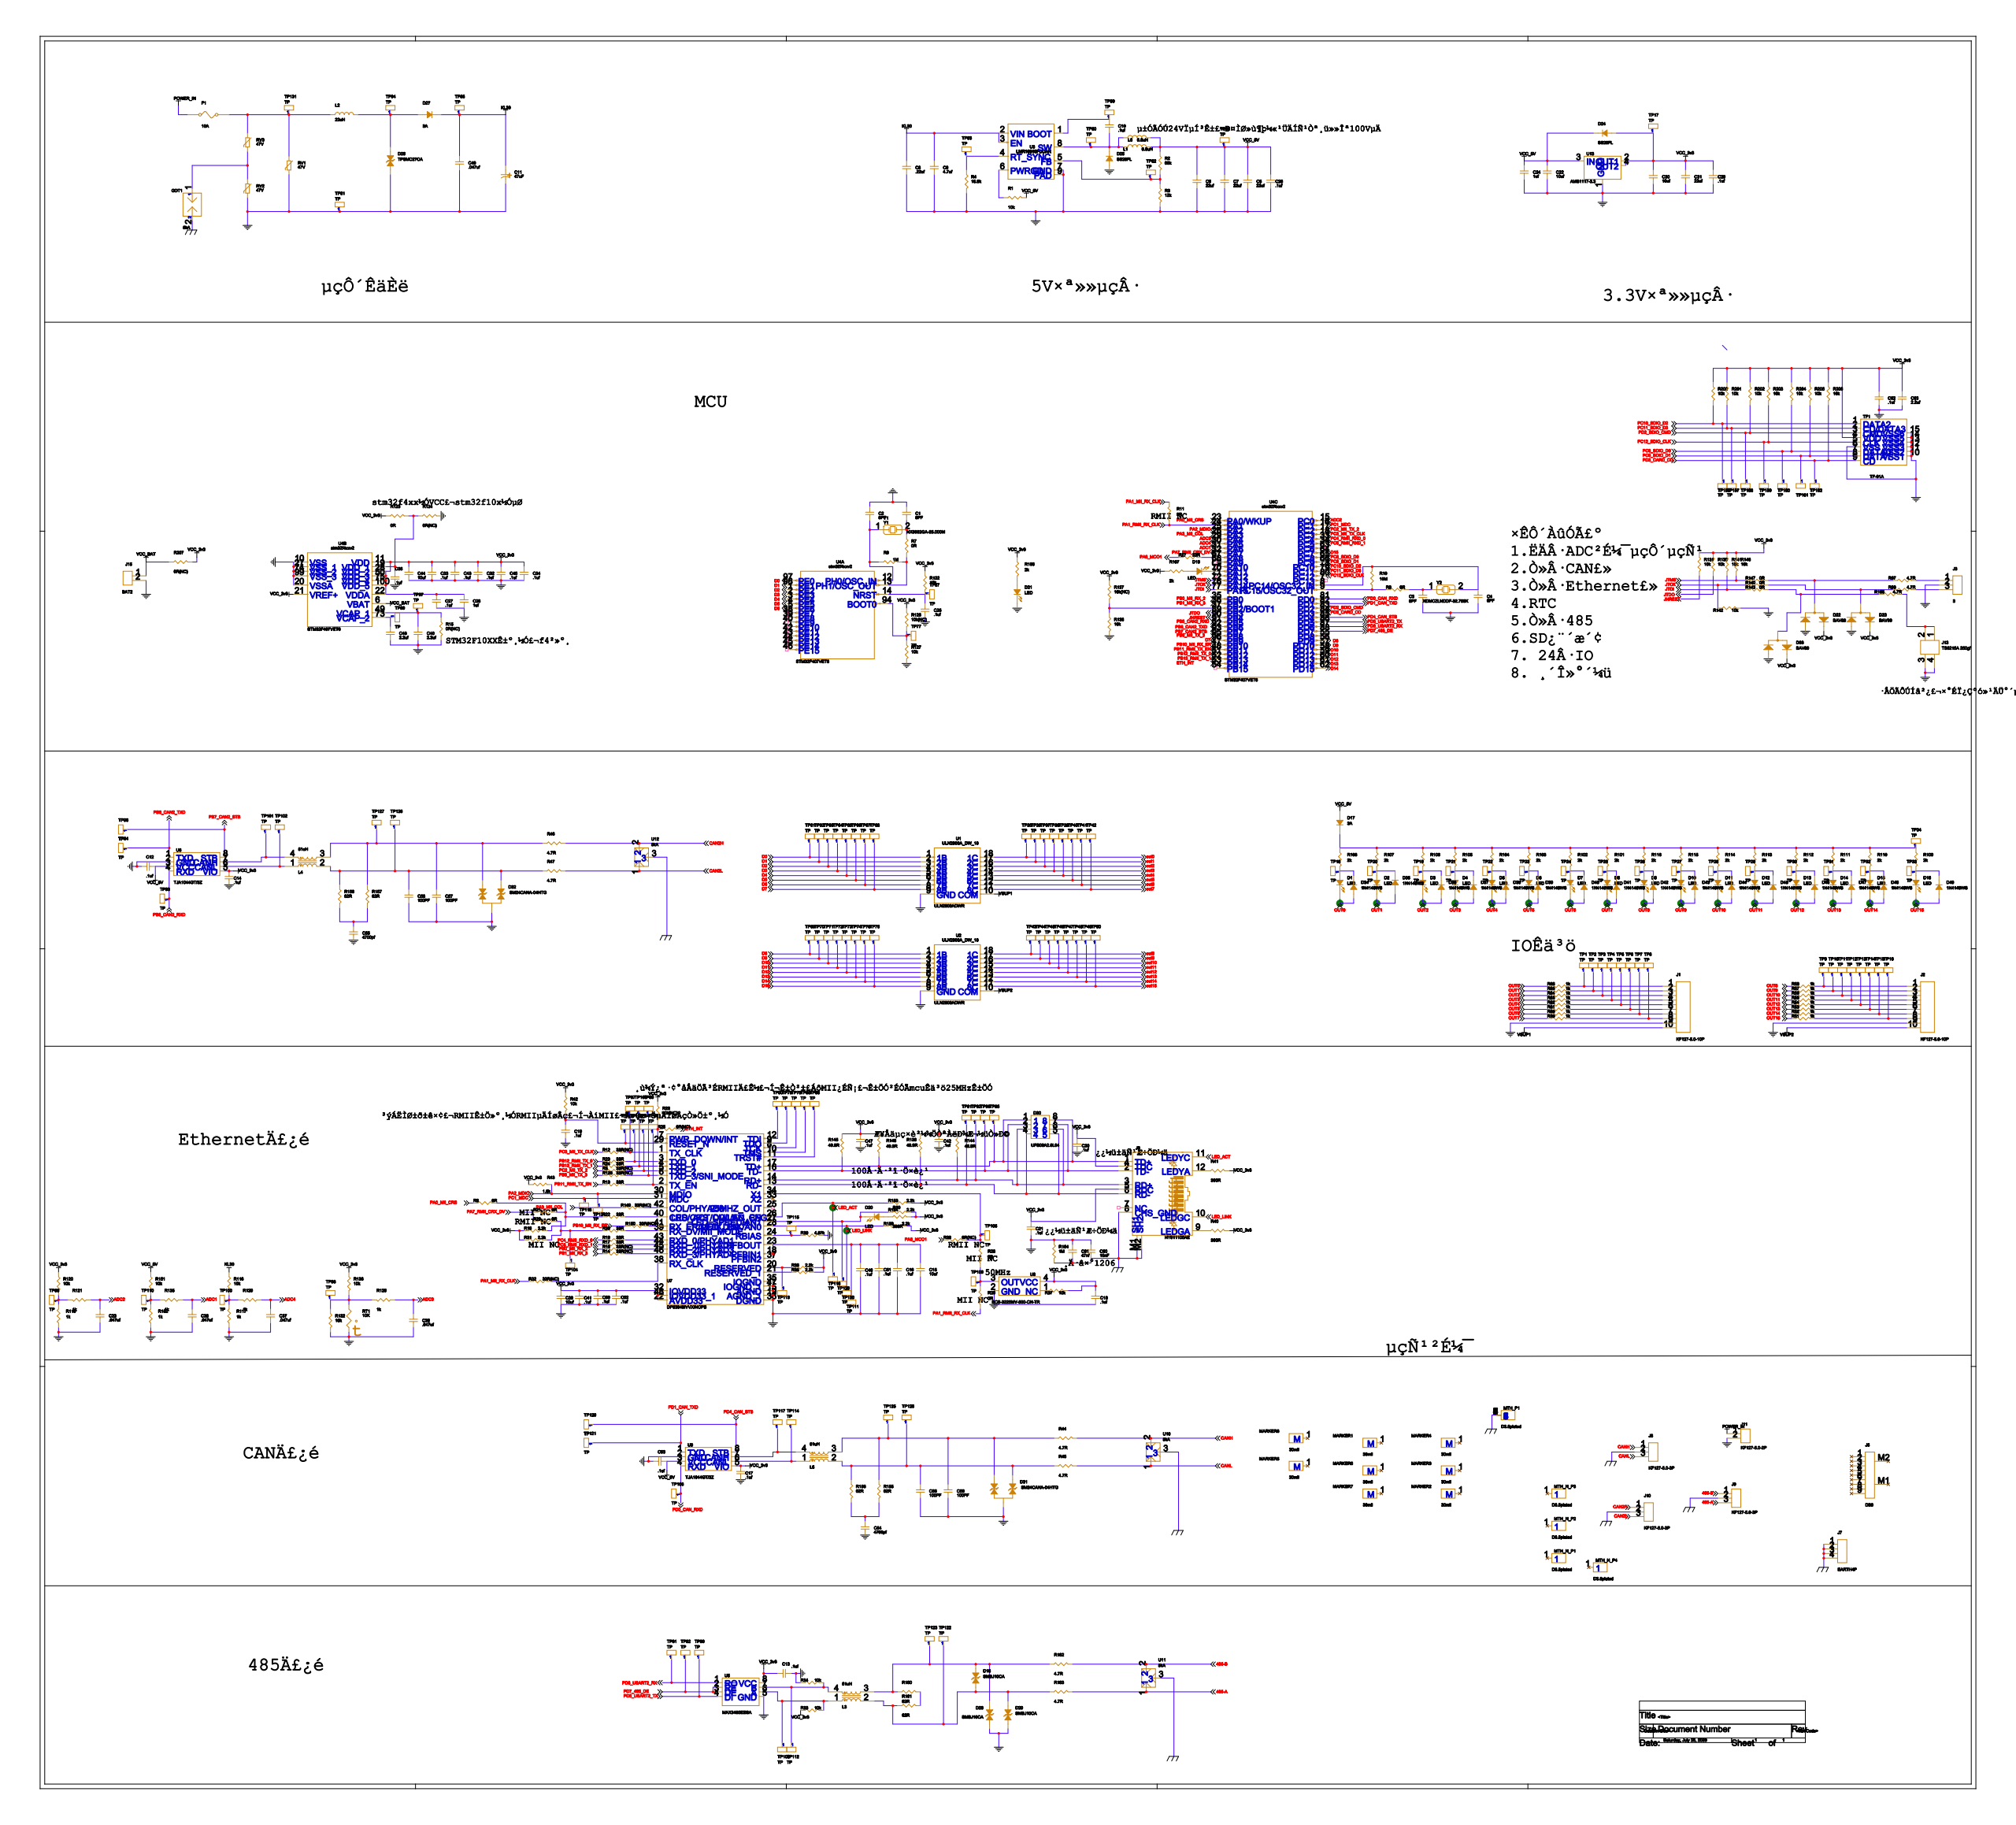Circuit board | Cadence Allegro | 429 parts | 215 nets
Bill of materials:
SYM_NAME,COMP_DEVICE_TYPE,COMP_VALUE,COMP_TOL,COMP_CLASS,REFDES
C0402,CAP_NP_C0402_8PF,8PF,,IC,C1
C0402,CAP_NP_C0402_8PF,8PF,,IC,C2
C0402,CAP_NP_C0402_6PF,6PF,,IC,C3
C0402,CAP_NP_C0402_6PF,6PF,,IC,C4
C1210,CAP_NP_C1210_22UF,22uf,,IC,C5
C1210,CAP_NP_C1210_22UF,22uf,,IC,C6
C1210,CAP_NP_C1210_22UF,22uf,,IC,C7
C0805,CAP_NP_C0805_.22UF,.22uf,,IC,C8
C1210,CAP_NP_C1210_4.7UF,4.7uf,,IC,C9
C0402,CAP_NP_C0402_.1UF,.1uf,,IC,C10
CAPAE630X770N,CAP_POL_CAPAE630X770N_47UF,47uF,,IC,C11
C0402,CAP_NP_C0402_.1UF,.1uf,,IC,C12
C0402,CAP_NP_C0402_.1UF,.1uf,,IC,C13
C0402,CAP_NP_C0402_.1UF,.1uf,,IC,C14
C1210,CAP_NP_C1210_10UF,10uf,,IC,C15
C0402,CAP_NP_C0402_.1UF,.1uf,,IC,C16
C0402,CAP_NP_C0402_.1UF,.1uf,,IC,C17
C0402,CAP_NP_C0402_.1UF,.1uf,,IC,C18
C0402,CAP_NP_C0402_.1UF,.1uf,,IC,C19
C0402,CAP_NP_C0402_.1UF,.1uf,,IC,C20
C0402,CAP_NP_C0402_.1UF,.1uf,,IC,C21
C1210,CAP_NP_C1210_10UF,10uf,,IC,C22
C0402,CAP_NP_C0402_.047UF,.047uf,,IC,C23
C0603,CAP_NP_C0603_1UF,1uf,,IC,C24
C0402,CAP_NP_C0402_.1UF,.1uf,,IC,C25
C0402,CAP_NP_C0402_.1UF,.1uf,,IC,C26
C0402,CAP_NP_C0402_.1UF,.1uf,,IC,C27
C0603,CAP_NP_C0603_1UF,1uf,,IC,C28
C0402,CAP_NP_C0402_.1UF,.1uf,,IC,C29
C1210,CAP_NP_C1210_10UF,10uf,,IC,C30
C1210,CAP_NP_C1210_22UF,22uf,,IC,C31
C0402,CAP_NP_C0402_.1UF,.1uf,,IC,C32
C0402,CAP_NP_C0402_.1UF,.1uf,,IC,C33
C0402,CAP_NP_C0402_.1UF,.1uf,,IC,C34
C0402,CAP_NP_C0402_.1UF,.1uf,,IC,C35
C0402,CAP_NP_C0402_.047UF,.047uf,,IC,C36
C0402,CAP_NP_C0402_.047UF,.047uf,,IC,C37
C0402,CAP_NP_C0402_.047UF,.047uf,,IC,C38
C1210,CAP_NP_C1210_10UF,10uf,,IC,C39
C0603,CAP_NP_C0603_2.2UF,2.2uf,,IC,C40
C0402,CAP_NP_C0402_.1UF,.1uf,,IC,C41
C0402,CAP_NP_C0402_.1UF,.1uf,,IC,C42
C0402,CAP_NP_C0402_.1UF,.1uf,,IC,C43
C1210,CAP_NP_C1210_10UF,10uf,,IC,C44
C0402,CAP_NP_C0402_.1UF,.1uf,,IC,C45
C0402,CAP_NP_C0402_.1UF,.1uf,,IC,C46
C0402,CAP_NP_C0402_.1UF,.1uf,,IC,C47
C0603,CAP_NP_C0603_2.2UF,2.2uf,,IC,C48
C0805,CAP_NP_C0805_.047UF,.047uf,,IC,C49
C0402,CAP_NP_C0402_.1UF,.1uf,,IC,C50
C0402,CAP_NP_C0402_.1UF,.1uf,,IC,C51
C0402,CAP_NP_C0402_.1UF,.1uf,,IC,C52
C0402,CAP_NP_C0402_.1UF,.1uf,,IC,C53
C0603,CAP_NP_C0603_4700PF,4700pf,,IC,C54
C0603,CAP_NP_C0603_4700PF,4700pf,,IC,C55
C0603,CAP_NP_C0603_100PF,100PF,,IC,C56
C0603,CAP_NP_C0603_100PF,100PF,,IC,C57
C0603,CAP_NP_C0603_100PF,100PF,,IC,C58
C0603,CAP_NP_C0603_100PF,100PF,,IC,C59
C1206,CAP_NP_C1206_10NF,10nF,,IC,C60
C1210,CAP_NP_C1210_47NF,47nf,,IC,C61
C0402,CAP_NP_C0402_.1UF,.1uf,,IC,C62
C0603,CAP_NP_C0603_2.2UF,2.2uf,,IC,C63
LEDRR254,LED_LEDRR254_LED,LED,,IC,D1
LEDRR254,LED_LEDRR254_LED,LED,,IC,D2
LEDRR254,LED_LEDRR254_LED,LED,,IC,D3
LEDRR254,LED_LEDRR254_LED,LED,,IC,D4
LEDRR254,LED_LEDRR254_LED,LED,,IC,D5
LEDRR254,LED_LEDRR254_LED,LED,,IC,D6
LEDRR254,LED_LEDRR254_LED,LED,,IC,D7
LEDRR254,LED_LEDRR254_LED,LED,,IC,D8
LEDRR254,LED_LEDRR254_LED,LED,,IC,D9
LEDRR254,LED_LEDRR254_LED,LED,,IC,D10
LEDRR254,LED_LEDRR254_LED,LED,,IC,D11
LEDRR254,LED_LEDRR254_LED,LED,,IC,D12
LEDRR254,LED_LEDRR254_LED,LED,,IC,D13
LEDRR254,LED_LEDRR254_LED,LED,,IC,D14
LEDRR254,LED_LEDRR254_LED,LED,,IC,D15
LEDRR254,LED_LEDRR254_LED,LED,,IC,D16
SMB,DIODE_SMB_3A,3A,,IC,D17
SMB,TVS_BI_SMB_SMBJ10CA,SMBJ10CA,,IC,D18
LEDRR254,LED_LEDRR254_LED,LED,,IC,D19
LEDRR254,LED_LEDRR254_LED,LED,,IC,D20
LEDRR254,LED_LEDRR254_LED,LED,,IC,D21
SOT-23,BAV99_SOT-23_BAV99,BAV99,,IC,D22
SOT-23,BAV99_SOT-23_BAV99,BAV99,,IC,D23
SMA,DIODE_SMA_SS26FL,SS26FL,,IC,D24
SMA,DIODE_SMA_SS26FL,SS26FL,,IC,D25
SMC,TVS_BI_SMC_TPSMC27CA,TPSMC27CA,,IC,D26
SMB,DIODE_SMB_3A,3A,,IC,D27
SMB,TVS_BI_SMB_SMBJ10CA,SMBJ10CA,,IC,D28
SMB,TVS_BI_SMB_SMBJ10CA,SMBJ10CA,,IC,D29
SOIC127P600X175-8N,ETH_TVS_SOIC127P600X175-8N_UFS0,UFS08A2.8L04,,IC,D30
SOT23,CAN_TVS_SOT23_ SM24CANA-04HTG,SM24CANA-04HTG,,IC,D31
SOT23,CAN_TVS_SOT23_ SM24CANA-04HTG,SM24CANA-04HTG,,IC,D32
SOT-23,BAV99_SOT-23_BAV99,BAV99,,IC,D33
SOD-323,DIODE_SOD-323_1N4148WS,1N4148WS,,IC,D34
SOD-323,DIODE_SOD-323_1N4148WS,1N4148WS,,IC,D35
SOD-323,DIODE_SOD-323_1N4148WS,1N4148WS,,IC,D36
SOD-323,DIODE_SOD-323_1N4148WS,1N4148WS,,IC,D37
SOD-323,DIODE_SOD-323_1N4148WS,1N4148WS,,IC,D38
SOD-323,DIODE_SOD-323_1N4148WS,1N4148WS,,IC,D39
SOD-323,DIODE_SOD-323_1N4148WS,1N4148WS,,IC,D40
SOD-323,DIODE_SOD-323_1N4148WS,1N4148WS,,IC,D41
SOD-323,DIODE_SOD-323_1N4148WS,1N4148WS,,IC,D42
SOD-323,DIODE_SOD-323_1N4148WS,1N4148WS,,IC,D43
SOD-323,DIODE_SOD-323_1N4148WS,1N4148WS,,IC,D44
SOD-323,DIODE_SOD-323_1N4148WS,1N4148WS,,IC,D45
SOD-323,DIODE_SOD-323_1N4148WS,1N4148WS,,IC,D46
SOD-323,DIODE_SOD-323_1N4148WS,1N4148WS,,IC,D47
SOD-323,DIODE_SOD-323_1N4148WS,1N4148WS,,IC,D48
SOD-323,DIODE_SOD-323_1N4148WS,1N4148WS,,IC,D49
FUSE10A,FUSE_FUSE10A_10A,10A,,IC,F1
GDT5KA2P,GDT_GDT5KA2P_5KA,5kA,,IC,GDT1
PHONEX10P500_82,CON10_PHONEX10P500_82_KF127-5.0,KF127-5.0-10P,,IC,J1
PHONEX10P500_82,CON10_PHONEX10P500_82_KF127-5.0,KF127-5.0-10P,,IC,J2
PHONEX3P500,CON3_PHONEX3P500_3,3,,IC,J3
DB_V_R-9,DB9_DB_V_R-9_DB9,DB9,,IC,J5
RJ_RA-8,HY911105AE_RJ_RA-8_IO_HY911105A,HY911105AE,,IO,J6
EARTH4P_M3,EARTH4P_EARTH4P_M3_EARTH4P,EARTH4P,,IC,J7
PHONEX3P500_82,CON3_PHONEX3P500_82_KF127-5.0-3,KF127-5.0-3P,,IC,J8
PHONEX3P500_82,CON3_PHONEX3P500_82_KF127-5.0-3,KF127-5.0-3P,,IC,J9
PHONEX3P500_82,CON3_PHONEX3P500_82_KF127-5.0-3,KF127-5.0-3P,,IC,J10
PHONEX2P500_82,CON2_PHONEX2P500_82_KF127-5.0-2,KF127-5.0-2P,,IC,J11
TS5215A,TC_TS5215A_TS5215A 250GF,TS5215A 250gf,,IC,J13
CR1220,CON2_CR1220_BAT2,BAT2,,IC,J15
SPM5030,INDUCTOR_SPM5030_6.8UH,6.8uH,,IC,L1
SPM6530,INDUCTOR_SPM6530_22UH,22uH,,IC,L2
CM320X450X150-4N,CHOKE CM14_CM320X450X150-4N_51U,51uH,,IC,L3
CM320X450X150-4N,CHOKE CM14_CM320X450X150-4N_51U,51uH,,IC,L4
CM320X450X150-4N,CHOKE CM14_CM320X450X150-4N_51U,51uH,,IC,L5
SNR5040,INDUCTOR_SNR5040_6.8UH,6.8uH,,IC,L6
FIDMS0,MARKER_FIDMS0_30MIL,30mil,,IC,MARKER1
FIDMS0,MARKER_FIDMS0_30MIL,30mil,,IC,MARKER2
FIDMS0,MARKER_FIDMS0_30MIL,30mil,,IC,MARKER3
FIDMS0,MARKER_FIDMS0_30MIL,30mil,,IC,MARKER4
FIDMS0,MARKER_FIDMS0_30MIL,30mil,,IC,MARKER5
FIDMS0,MARKER_FIDMS0_30MIL,30mil,,IC,MARKER6
FIDMS0,MARKER_FIDMS0_30MIL,30mil,,IC,MARKER7
FIDMS0,MARKER_FIDMS0_30MIL,30mil,,IC,MARKER8
MTGP770H350P,MTH_NO_PLATED_MTGP770H350P_D3.5,D3.5plated,,IC,MTH_N_P1
MTGP770H350P,MTH_NO_PLATED_MTGP770H350P_D3.5,D3.5plated,,IC,MTH_N_P2
MTGP770H350P,MTH_NO_PLATED_MTGP770H350P_D3.5,D3.5plated,,IC,MTH_N_P3
MTGP770H350P,MTH_NO_PLATED_MTGP770H350P_D3.5,D3.5plated,,IC,MTH_N_P4
MTGP770H350V6P,MTH_PLATED_MTGP770H350V6P_D3.5P,D3.5plated,,IC,MTH_P1
R0402,R0402_R0402_10K,10k,,DISCRETE,R1
R0402,R0402_R0402_68K,68k,,IC,R2
R0402,R0402_R0402_12K,12k,,IC,R3
R0402,R0402_R0402_16.9K,16.9k,,IC,R4
R0402,R0402_R0402_33R(NC),33R(NC),,DISCRETE,R5
R0402,R0402_R0402_0R,0R,,DISCRETE,R6
R0402,R0402_R0402_0R,0R,,DISCRETE,R7
R0402,R0402_R0402_0R,0R,,DISCRETE,R8
R0402,R0402_R0402_1M,1M,,IC,R9
R0402,R0402_R0402_10M,10M,,IC,R10
R0402,R0402_R0402_0R,0R,,DISCRETE,R11
R0402,R0402_R0402_33R(NC),33R(NC),,DISCRETE,R12
R0402,R0402_R0402_33R,33R,,DISCRETE,R13
R0402,R0402_R0402_33R(NC),33R(NC),,DISCRETE,R14
R0402,R0402_R0402_0R(NC),0R(NC),,IC,R15
R0402,R0402_R0402_33R(NC),33R(NC),,DISCRETE,R16
R0402,R0402_R0402_33R,33R,,DISCRETE,R17
R0402,R0402_R0402_2.2K,2.2k,,IC,R18
R0402,R0402_R0402_33R,33R,,DISCRETE,R19
R0402,R0402_R0402_0R,0R,,DISCRETE,R20
R0402,R0402_R0402_0R,0R,,DISCRETE,R21
R0402,R0402_R0402_33R,33R,,DISCRETE,R22
R0402,R0402_R0402_33R,33R,,DISCRETE,R23
R0402,R0402_R0402_33R,33R,,DISCRETE,R24
R0402,R0402_R0402_0R(NC),0R(NC),,IC,R25
R0402,R0402_R0402_10K(NC),10k(NC),,IC,R26
R0402,R0402_R0402_33R,33R,,DISCRETE,R27
R0402,R0402_R0402_0R,0R,,DISCRETE,R28
R0402,R0402_R0402_0R,0R,,DISCRETE,R29
R0402,R0402_R0402_33R,33R,,DISCRETE,R30
R0402,R0402_R0402_2.2K,2.2k,,IC,R31
R0402,R0402_R0402_33R(NC),33R(NC),,DISCRETE,R32
R0402,R0402_R0402_10K,10k,,DISCRETE,R33
R0402,R0402_R0402_10K,10k,,DISCRETE,R34
R0402,R0402_R0402_2.2K,2.2k,,IC,R35
R0402,R0402_R0402_2.2K,2.2k,,IC,R36
R0402,R0402_R0402_10K,10k,,DISCRETE,R37
R0402,R0402_R0402_0R(NC),0R(NC),,IC,R38
R0402,R0402_R0402_4.87K,4.87k,,IC,R39
R0805,R0805_R0805_390R,390R,,IC,R40
R0805,R0805_R0805_390R,390R,,IC,R41
R0402,R0402_R0402_10K,10k,,DISCRETE,R42
R0402,R0402_R0402_1.5K,1.5k,,IC,R43
R1206,R1206_R1206_4.7R,4.7R,,IC,R44
R1206,R1206_R1206_4.7R,4.7R,,IC,R45
R1206,R1206_R1206_4.7R,4.7R,,IC,R46
R1206,R1206_R1206_4.7R,4.7R,,IC,R47
R0805,R0805_R0805_390R,390R,,IC,R50
R0805,R0805_R0805_1K,1k,,IC,R51
R0805,R0805_R0805_1K,1k,,IC,R52
R0805,R0805_R0805_1K,1k,,IC,R53
R0805,R0805_R0805_1K,1k,,IC,R54
R0805,R0805_R0805_1K,1k,,IC,R55
R0805,R0805_R0805_1K,1k,,IC,R56
R0805,R0805_R0805_1K,1k,,IC,R57
R0805,R0805_R0805_1K,1k,,IC,R58
R0805,R0805_R0805_1K,1k,,IC,R59
R0805,R0805_R0805_1K,1k,,IC,R60
R0805,R0805_R0805_1K,1k,,IC,R61
R0805,R0805_R0805_1K,1k,,IC,R62
R0805,R0805_R0805_1K,1k,,IC,R63
R0805,R0805_R0805_1K,1k,,IC,R64
R0805,R0805_R0805_1K,1k,,IC,R65
R0805,R0805_R0805_1K,1k,,IC,R66
R1206,R1206_R1206_4.7R,4.7R,,IC,R67
R1206,R1206_R1206_4.7R,4.7R,,IC,R68
R0805,R0805_R0805_2K,2k,,IC,R101
R0805,R0805_R0805_2K,2k,,IC,R102
R0805,R0805_R0805_2K,2k,,IC,R103
R0805,R0805_R0805_2K,2k,,IC,R104
R0805,R0805_R0805_2K,2k,,IC,R105
R0805,R0805_R0805_2K,2k,,IC,R106
R0805,R0805_R0805_2K,2k,,IC,R107
R0805,R0805_R0805_2K,2k,,IC,R108
R0805,R0805_R0805_2K,2k,,IC,R109
R0805,R0805_R0805_2K,2k,,IC,R110
R0805,R0805_R0805_2K,2k,,IC,R111
R0805,R0805_R0805_2K,2k,,IC,R112
R0805,R0805_R0805_2K,2k,,IC,R113
R0805,R0805_R0805_2K,2k,,IC,R114
R0805,R0805_R0805_2K,2k,,IC,R115
R0805,R0805_R0805_2K,2k,,IC,R116
R0402,R0402_R0402_1K,1k,,IC,R117
R0402,R0402_R0402_10K,10k,,DISCRETE,R118
R0402,R0402_R0402_1K,1k,,IC,R119
R0402,R0402_R0402_10K,10k,,DISCRETE,R120
R0402,R0402_R0402_1K,1k,,IC,R121
R0402,R0402_R0402_10K,10k,,DISCRETE,R122
R0402,R0402_R0402_0R,0R,,DISCRETE,R123
R0402,R0402_R0402_0R(NC),0R(NC),,IC,R124
R0402,R0402_R0402_10K(NC),10k(NC),,IC,R125
R0402,R0402_R0402_1K,1k,,IC,R126
R0402,R0402_R0402_10K,10k,,DISCRETE,R127
R0402,R0402_R0402_33R(NC),33R(NC),,DISCRETE,R128
R0402,R0402_R0402_1K,1k,,IC,R129
R0402,R0402_R0402_10K,10k,,DISCRETE,R130
R0402,R0402_R0402_10K,10k,,DISCRETE,R131
R0402,R0402_R0402_10K,10k,,DISCRETE,R132
R0402,R0402_R0402_1K,1k,,IC,R135
R0402,R0402_R0402_10K,10k,,DISCRETE,R136
R0402,R0402_R0402_10K(NC),10k(NC),,IC,R137
R0402,R0402_R0402_10K,10k,,DISCRETE,R138
R0603,R0603_R0603_49.9R,49.9R,,IC,R139
R0402,R0402_R0402_0R,0R,,DISCRETE,R140
R0402,R0402_R0402_10K,10k,,DISCRETE,R141
R0402,R0402_R0402_10K,10k,,DISCRETE,R142
R0402,R0402_R0402_0R,0R,,DISCRETE,R143
R0603,R0603_R0603_49.9R,49.9R,,IC,R144
R0603,R0603_R0603_49.9R,49.9R,,IC,R145
R0402,R0402_R0402_10K,10k,,DISCRETE,R146
R0402,R0402_R0402_0R,0R,,DISCRETE,R147
R0603,R0603_R0603_49.9R,49.9R,,IC,R148
R0402,R0402_R0402_33R(NC),33R(NC),,DISCRETE,R149
R0402,R0402_R0402_33R(NC),33R(NC),,DISCRETE,R150
R0402,R0402_R0402_10K,10k,,DISCRETE,R151
R0402,R0402_R0402_1K,1k,,IC,R152
R0402,R0402_R0402_2.2K,2.2k,,IC,R153
R0402,R0402_R0402_2.2K,2.2k,,IC,R154
R1206,R1206_R1206_62R,62R,,IC,R155
R1206,R1206_R1206_62R,62R,,IC,R156
R1206,R1206_R1206_62R,62R,,IC,R157
R1206,R1206_R1206_62R,62R,,IC,R158
R0402,R0402_R0402_2.2K,2.2k,,IC,R159
R1206,R1206_R1206_62R,62R,,IC,R160
R1206,R1206_R1206_62R,62R,,IC,R161
R1206,R1206_R1206_4.7R,4.7R,,IC,R162
R1206,R1206_R1206_4.7R,4.7R,,IC,R163
R1206,R1206_R1206_1M,1M,,IC,R164
R1206,R1206_R1206_4.7R,4.7R,,IC,R165
R0805,R0805_R0805_2K,2k,,IC,R166
R0805,R0805_R0805_2K,2k,,IC,R167
R0402,R0402_R0402_10K,10k,,DISCRETE,R200
R0402,R0402_R0402_10K,10k,,DISCRETE,R201
R0402,R0402_R0402_10K,10k,,DISCRETE,R202
R0402,R0402_R0402_10K,10k,,DISCRETE,R203
R0402,R0402_R0402_10K,10k,,DISCRETE,R204
R0402,R0402_R0402_10K,10k,,DISCRETE,R205
R0402,R0402_R0402_10K,10k,,DISCRETE,R206
R0402,R0402_R0402_0R(NC),0R(NC),,IC,R207
R0603,THERMISTOR_R0603_10K,10K,,IC,RT1
R2220,VARISTOR SYM_R2220_47V,47V,,IC,RV1
R2220,VARISTOR SYM_R2220_47V,47V,,IC,RV2
R2220,VARISTOR SYM_R2220_47V,47V,,IC,RV3
TF-01A,TF_TF-01A_TF-01A,TF-01A,,IC,TF1
TPAD_30MIL,TP_TPAD_30MIL_TP,TP,,DISCRETE,TP1
TPAD_30MIL,TP_TPAD_30MIL_TP,TP,,DISCRETE,TP2
TPAD_30MIL,TP_TPAD_30MIL_TP,TP,,DISCRETE,TP3
TPAD_30MIL,TP_TPAD_30MIL_TP,TP,,DISCRETE,TP4
TPAD_30MIL,TP_TPAD_30MIL_TP,TP,,DISCRETE,TP5
TPAD_30MIL,TP_TPAD_30MIL_TP,TP,,DISCRETE,TP6
TPAD_30MIL,TP_TPAD_30MIL_TP,TP,,DISCRETE,TP7
TPAD_30MIL,TP_TPAD_30MIL_TP,TP,,DISCRETE,TP8
TPAD_30MIL,TP_TPAD_30MIL_TP,TP,,DISCRETE,TP9
TPAD_30MIL,TP_TPAD_30MIL_TP,TP,,DISCRETE,TP10
TPAD_30MIL,TP_TPAD_30MIL_TP,TP,,DISCRETE,TP11
TPAD_30MIL,TP_TPAD_30MIL_TP,TP,,DISCRETE,TP12
TPAD_30MIL,TP_TPAD_30MIL_TP,TP,,DISCRETE,TP13
TPAD_30MIL,TP_TPAD_30MIL_TP,TP,,DISCRETE,TP14
TPAD_30MIL,TP_TPAD_30MIL_TP,TP,,DISCRETE,TP15
TPAD_30MIL,TP_TPAD_30MIL_TP,TP,,DISCRETE,TP16
TPAD_30MIL,TP_TPAD_30MIL_TP,TP,,DISCRETE,TP17
TPAD_30MIL,TP_TPAD_30MIL_TP,TP,,DISCRETE,TP18
TPAD_30MIL,TP_TPAD_30MIL_TP,TP,,DISCRETE,TP19
TPAD_30MIL,TP_TPAD_30MIL_TP,TP,,DISCRETE,TP20
TPAD_30MIL,TP_TPAD_30MIL_TP,TP,,DISCRETE,TP21
TPAD_30MIL,TP_TPAD_30MIL_TP,TP,,DISCRETE,TP22
TPAD_30MIL,TP_TPAD_30MIL_TP,TP,,DISCRETE,TP23
TPAD_30MIL,TP_TPAD_30MIL_TP,TP,,DISCRETE,TP24
TPAD_30MIL,TP_TPAD_30MIL_TP,TP,,DISCRETE,TP25
TPAD_30MIL,TP_TPAD_30MIL_TP,TP,,DISCRETE,TP26
TPAD_30MIL,TP_TPAD_30MIL_TP,TP,,DISCRETE,TP27
TPAD_30MIL,TP_TPAD_30MIL_TP,TP,,DISCRETE,TP28
TPAD_30MIL,TP_TPAD_30MIL_TP,TP,,DISCRETE,TP29
TPAD_30MIL,TP_TPAD_30MIL_TP,TP,,DISCRETE,TP30
TPAD_30MIL,TP_TPAD_30MIL_TP,TP,,DISCRETE,TP31
TPAD_30MIL,TP_TPAD_30MIL_TP,TP,,DISCRETE,TP32
TPAD_30MIL,TP_TPAD_30MIL_TP,TP,,DISCRETE,TP33
TPAD_30MIL,TP_TPAD_30MIL_TP,TP,,DISCRETE,TP34
TPAD_30MIL,TP_TPAD_30MIL_TP,TP,,DISCRETE,TP35
TPAD_30MIL,TP_TPAD_30MIL_TP,TP,,DISCRETE,TP36
TPAD_30MIL,TP_TPAD_30MIL_TP,TP,,DISCRETE,TP37
TPAD_30MIL,TP_TPAD_30MIL_TP,TP,,DISCRETE,TP38
TPAD_30MIL,TP_TPAD_30MIL_TP,TP,,DISCRETE,TP39
TPAD_30MIL,TP_TPAD_30MIL_TP,TP,,DISCRETE,TP40
TPAD_30MIL,TP_TPAD_30MIL_TP,TP,,DISCRETE,TP41
TPAD_30MIL,TP_TPAD_30MIL_TP,TP,,DISCRETE,TP42
TPAD_30MIL,TP_TPAD_30MIL_TP,TP,,DISCRETE,TP43
TPAD_30MIL,TP_TPAD_30MIL_TP,TP,,DISCRETE,TP44
TPAD_30MIL,TP_TPAD_30MIL_TP,TP,,DISCRETE,TP45
TPAD_30MIL,TP_TPAD_30MIL_TP,TP,,DISCRETE,TP46
TPAD_30MIL,TP_TPAD_30MIL_TP,TP,,DISCRETE,TP47
TPAD_30MIL,TP_TPAD_30MIL_TP,TP,,DISCRETE,TP48
TPAD_30MIL,TP_TPAD_30MIL_TP,TP,,DISCRETE,TP49
TPAD_30MIL,TP_TPAD_30MIL_TP,TP,,DISCRETE,TP50
TPAD_30MIL,TP_TPAD_30MIL_TP,TP,,DISCRETE,TP51
TPAD_30MIL,TP_TPAD_30MIL_TP,TP,,DISCRETE,TP52
TPAD_30MIL,TP_TPAD_30MIL_TP,TP,,DISCRETE,TP53
TPAD_30MIL,TP_TPAD_30MIL_TP,TP,,DISCRETE,TP54
TPAD_30MIL,TP_TPAD_30MIL_TP,TP,,DISCRETE,TP55
TPAD_30MIL,TP_TPAD_30MIL_TP,TP,,DISCRETE,TP56
TPAD_30MIL,TP_TPAD_30MIL_TP,TP,,DISCRETE,TP57
TPAD_30MIL,TP_TPAD_30MIL_TP,TP,,DISCRETE,TP58
TPAD_30MIL,TP_TPAD_30MIL_TP,TP,,DISCRETE,TP59
TPAD_30MIL,TP_TPAD_30MIL_TP,TP,,DISCRETE,TP60
TPAD_30MIL,TP_TPAD_30MIL_TP,TP,,DISCRETE,TP61
TPAD_30MIL,TP_TPAD_30MIL_TP,TP,,DISCRETE,TP62
TPAD_30MIL,TP_TPAD_30MIL_TP,TP,,DISCRETE,TP63
TPAD_30MIL,TP_TPAD_30MIL_TP,TP,,DISCRETE,TP64
TPAD_30MIL,TP_TPAD_30MIL_TP,TP,,DISCRETE,TP65
TPAD_30MIL,TP_TPAD_30MIL_TP,TP,,DISCRETE,TP66
TPAD_30MIL,TP_TPAD_30MIL_TP,TP,,DISCRETE,TP67
TPAD_30MIL,TP_TPAD_30MIL_TP,TP,,DISCRETE,TP68
TPAD_30MIL,TP_TPAD_30MIL_TP,TP,,DISCRETE,TP69
TPAD_30MIL,TP_TPAD_30MIL_TP,TP,,DISCRETE,TP70
TPAD_30MIL,TP_TPAD_30MIL_TP,TP,,DISCRETE,TP71
TPAD_30MIL,TP_TPAD_30MIL_TP,TP,,DISCRETE,TP72
TPAD_30MIL,TP_TPAD_30MIL_TP,TP,,DISCRETE,TP73
TPAD_30MIL,TP_TPAD_30MIL_TP,TP,,DISCRETE,TP74
TPAD_30MIL,TP_TPAD_30MIL_TP,TP,,DISCRETE,TP75
TPAD_30MIL,TP_TPAD_30MIL_TP,TP,,DISCRETE,TP76
TPAD_30MIL,TP_TPAD_30MIL_TP,TP,,DISCRETE,TP77
TPAD_30MIL,TP_TPAD_30MIL_TP,TP,,DISCRETE,TP78
TPAD_30MIL,TP_TPAD_30MIL_TP,TP,,DISCRETE,TP79
TPAD_30MIL,TP_TPAD_30MIL_TP,TP,,DISCRETE,TP80
TPAD_30MIL,TP_TPAD_30MIL_TP,TP,,DISCRETE,TP81
TPAD_30MIL,TP_TPAD_30MIL_TP,TP,,DISCRETE,TP82
TPAD_30MIL,TP_TPAD_30MIL_TP,TP,,DISCRETE,TP83
TPAD_30MIL,TP_TPAD_30MIL_TP,TP,,DISCRETE,TP84
TPAD_30MIL,TP_TPAD_30MIL_TP,TP,,DISCRETE,TP85
TPAD_30MIL,TP_TPAD_30MIL_TP,TP,,DISCRETE,TP86
TPAD_30MIL,TP_TPAD_30MIL_TP,TP,,DISCRETE,TP87
TPAD_30MIL,TP_TPAD_30MIL_TP,TP,,DISCRETE,TP88
TPAD_30MIL,TP_TPAD_30MIL_TP,TP,,DISCRETE,TP89
TPAD_30MIL,TP_TPAD_30MIL_TP,TP,,DISCRETE,TP90
TPAD_30MIL,TP_TPAD_30MIL_TP,TP,,DISCRETE,TP91
TPAD_30MIL,TP_TPAD_30MIL_TP,TP,,DISCRETE,TP92
TPAD_30MIL,TP_TPAD_30MIL_TP,TP,,DISCRETE,TP93
TPAD_30MIL,TP_TPAD_30MIL_TP,TP,,DISCRETE,TP94
TPAD_30MIL,TP_TPAD_30MIL_TP,TP,,DISCRETE,TP95
TPAD_30MIL,TP_TPAD_30MIL_TP,TP,,DISCRETE,TP96
TPAD_30MIL,TP_TPAD_30MIL_TP,TP,,DISCRETE,TP97
TPAD_30MIL,TP_TPAD_30MIL_TP,TP,,DISCRETE,TP98
TPAD_30MIL,TP_TPAD_30MIL_TP,TP,,DISCRETE,TP99
TPAD_30MIL,TP_TPAD_30MIL_TP,TP,,DISCRETE,TP100
TPAD_30MIL,TP_TPAD_30MIL_TP,TP,,DISCRETE,TP101
TPAD_30MIL,TP_TPAD_30MIL_TP,TP,,DISCRETE,TP102
TPAD_30MIL,TP_TPAD_30MIL_TP,TP,,DISCRETE,TP103
TPAD_30MIL,TP_TPAD_30MIL_TP,TP,,DISCRETE,TP104
TPAD_30MIL,TP_TPAD_30MIL_TP,TP,,DISCRETE,TP105
TPAD_30MIL,TP_TPAD_30MIL_TP,TP,,DISCRETE,TP106
TPAD_30MIL,TP_TPAD_30MIL_TP,TP,,DISCRETE,TP107
TPAD_30MIL,TP_TPAD_30MIL_TP,TP,,DISCRETE,TP108
TPAD_30MIL,TP_TPAD_30MIL_TP,TP,,DISCRETE,TP109
TPAD_30MIL,TP_TPAD_30MIL_TP,TP,,DISCRETE,TP110
TPAD_30MIL,TP_TPAD_30MIL_TP,TP,,DISCRETE,TP111
TPAD_30MIL,TP_TPAD_30MIL_TP,TP,,DISCRETE,TP112
TPAD_30MIL,TP_TPAD_30MIL_TP,TP,,DISCRETE,TP113
TPAD_30MIL,TP_TPAD_30MIL_TP,TP,,DISCRETE,TP114
TPAD_30MIL,TP_TPAD_30MIL_TP,TP,,DISCRETE,TP115
TPAD_30MIL,TP_TPAD_30MIL_TP,TP,,DISCRETE,TP116
TPAD_30MIL,TP_TPAD_30MIL_TP,TP,,DISCRETE,TP117
TPAD_30MIL,TP_TPAD_30MIL_TP,TP,,DISCRETE,TP118
TPAD_30MIL,TP_TPAD_30MIL_TP,TP,,DISCRETE,TP119
TPAD_30MIL,TP_TPAD_30MIL_TP,TP,,DISCRETE,TP120
TPAD_30MIL,TP_TPAD_30MIL_TP,TP,,DISCRETE,TP121
TPAD_30MIL,TP_TPAD_30MIL_TP,TP,,DISCRETE,TP122
TPAD_30MIL,TP_TPAD_30MIL_TP,TP,,DISCRETE,TP123
TPAD_30MIL,TP_TPAD_30MIL_TP,TP,,DISCRETE,TP124
TPAD_30MIL,TP_TPAD_30MIL_TP,TP,,DISCRETE,TP125
TPAD_30MIL,TP_TPAD_30MIL_TP,TP,,DISCRETE,TP126
TPAD_30MIL,TP_TPAD_30MIL_TP,TP,,DISCRETE,TP127
TPAD_30MIL,TP_TPAD_30MIL_TP,TP,,DISCRETE,TP128
TPAD_30MIL,TP_TPAD_30MIL_TP,TP,,DISCRETE,TP129
TPAD_30MIL,TP_TPAD_30MIL_TP,TP,,DISCRETE,TP130
TPAD_30MIL,TP_TPAD_30MIL_TP,TP,,DISCRETE,TP131
TPAD_30MIL,TP_TPAD_30MIL_TP,TP,,DISCRETE,TP156
TPAD_30MIL,TP_TPAD_30MIL_TP,TP,,DISCRETE,TP157
TPAD_30MIL,TP_TPAD_30MIL_TP,TP,,DISCRETE,TP158
TPAD_30MIL,TP_TPAD_30MIL_TP,TP,,DISCRETE,TP159
TPAD_30MIL,TP_TPAD_30MIL_TP,TP,,DISCRETE,TP160
TPAD_30MIL,TP_TPAD_30MIL_TP,TP,,DISCRETE,TP161
TPAD_30MIL,TP_TPAD_30MIL_TP,TP,,DISCRETE,TP162
DW18,ULN2803A_DW_18_DW18_ULN2803ADWR,ULN2803ADWR,,IC,U1
DW18,ULN2803A_DW_18_DW18_ULN2803ADWR,ULN2803ADWR,,IC,U2
DDA0008E_N,LMR16010PDDAR_DDA0008E_N_LMR160,LMR16010PDDAR,,IC,U3
LQFP100-14X14MM,STM32F4XXV2_LQFP100-14X14MM_STM,STM32F407VET6,,IC,U4
SOIC127P600X175-8N,SP485EEN-L/TR_SOIC127P600X175-8,MAX3485EESA,,IC,U5
SOIC127P600X175-8N,TJA1044GT/3Z_SOIC127P600X175-8N,TJA1044GT/3Z,,IC,U6
VBH48A_N,DP83848I_PT_48_VBH48A_N_DP83848,DP83848IVVX/NOPB,,IC,U7
OSCSC210P250X320X110-4N,Y_OSCSC210P250X320X110-4N_ECS-3,ECS-3225MV-500-CN-TR,,IC,U8
SOIC127P600X175-8N,TJA1044GT/3Z_SOIC127P600X175-8N,TJA1044GT/3Z,,IC,U9
GDT3P,GDTCM_GDT3P_5KA,5kA,,IC,U10
GDT3P,GDTCM_GDT3P_5KA,5kA,,IC,U11
GDT3P,GDTCM_GDT3P_5KA,5kA,,IC,U12
SOT223,AMS1117-3.3_SOT223_AMS1117-3.3,AMS1117-3.3,,IC,U13
XTAL500X320X150N,XTAL_XTAL500X320X150N_IC_NX5032,NX5032GA-25.000M,,IC,Y1
XTAL320X150X90N,XTAL_XTAL320X150X90N_IC_XDMCZLN,XDMCZLNDDF-32.768K,,IC,Y2
Netlist (net: part-pin ...):
N572960: D1-2 D34-1 R108-2 TP18-1
OUT0: D1-1 D34-2 R66-1 TP35-1 U1-18
N572931: D2-2 D35-1 R107-2 TP20-1
OUT1: D2-1 D35-2 R65-1 TP36-1 U1-17
N572924: D3-2 D36-1 R106-2 TP19-1
OUT2: D3-1 D36-2 R64-1 TP37-1 U1-16
N572897: D4-2 D37-1 R105-2 TP21-1
OUT3: D4-1 D37-2 R63-1 TP38-1 U1-15
N572890: D5-2 D38-1 R104-2 TP22-1
OUT4: D5-1 D38-2 R62-1 TP39-1 U1-14
N572863: D6-2 D39-1 R103-2 TP23-1
OUT5: D6-1 D39-2 R61-1 TP40-1 U1-13
N572856: D7-2 D40-1 R102-2 TP24-1
OUT6: D7-1 D40-2 R60-1 TP41-1 U1-12
N572829: D8-2 D41-1 R101-2 TP25-1
OUT7: D8-1 D41-2 R59-1 TP42-1 U1-11
N572812: D9-2 D42-1 R116-2 TP26-1
OUT8: D9-1 D42-2 R58-1 TP43-1 U2-18
N572793: D10-2 D43-1 R115-2 TP27-1
OUT9: D10-1 D43-2 R57-1 TP44-1 U2-17
N572776: D11-2 D44-1 R114-2 TP28-1
OUT10: D11-1 D44-2 R56-1 TP45-1 U2-16
N572769: D12-2 D45-1 R113-2 TP29-1
OUT11: D12-1 D45-2 R55-1 TP46-1 U2-15
N572752: D13-2 D46-1 R112-2 TP30-1
OUT12: D13-1 D46-2 R54-1 TP47-1 U2-14
N572735: D14-2 D47-1 R111-2 TP31-1
OUT13: D14-1 D47-2 R53-1 TP48-1 U2-13
N572710: D15-2 D48-1 R110-2 TP32-1
OUT14: D15-1 D48-2 R52-1 TP49-1 U2-12
N572699: D16-2 D49-1 R109-2 TP33-1
OUT15: D16-1 D49-2 R51-1 TP50-1 U2-11
N378187: J1-1 R66-2 TP1-1
VSUP1: J1-10 U1-10
N378264: J1-2 R65-2 TP2-1
N378301: J1-3 R64-2 TP3-1
N378341: J1-4 R63-2 TP4-1
N378381: J1-5 R62-2 TP5-1
N378420: J1-6 R61-2 TP6-1
N378459: J1-7 R60-2 TP7-1
N378498: J1-8 R59-2 TP8-1
GND: C1-1 C2-1 C3-2 C4-2 C5-2 C6-2 C7-2 C8-2 C9-2 C11-2 C12-1 C13-2 C14-2 C15-2 C16-2 C17-2 C18-2 C19-2 C20-2 C21-2 C22-2 C23-2 C24-2 C25-2 C26-2 C27-2 C28-2 C29-2 C30-2 C31-2 C32-2 C33-2 C34-2 C35-2 C36-2 C37-2 C38-2 C39-2 C40-2 C41-2 C42-2 C43-2 C44-2 C45-2 C46-2 C47-2 C48-2 C49-2 C50-2 C51-2 C52-2 C53-1 C54-2 C55-2 C56-2 C57-2 C58-2 C59-2 C60-1 C61-1 C62-2 C63-2 D21-1 D22-1 D23-1 D25-2 D26-1 D28-1 D29-1 D31-3 D32-3 D33-1 J1-9 J2-9 J3-2 J11-2 J13-3 J13-4 J15-2 R3-2 R4-2 R15-2 R34-1 R39-2 R117-1 R119-1 R124-2 R127-2 R132-2 R138-2 R142-2 R152-1 R164-1 RT1-2 RV1-2 RV2-2 TF1-6 TF1-10 TF1-11 TF1-12 TF1-13 TF1-14 TF1-15 TP51-1 U1-9 U2-9 U3-7 U3-9 U4-10 U4-20 U4-27 U4-74 U4-99 U5-5 U6-2 U7-15 U7-19 U7-35 U7-36 U7-47 U8-2 U9-2 U13-1
N380711: J2-1 R58-2 TP9-1
VSUP2: J2-10 U2-10
N380713: J2-2 R57-2 TP10-1
N380715: J2-3 R56-2 TP11-1
N380717: J2-4 R55-2 TP12-1
N380719: J2-5 R54-2 TP13-1
N380721: J2-6 R53-2 TP14-1
N380723: J2-7 R52-2 TP15-1
N380725: J2-8 R51-2 TP16-1
CAN2H: J10-1 R46-2 U12-2
GND_EARTH: C60-2 C61-2 GDT1-2 J6-8 J6-M1 J6-M2 J7-1 J7-2 J7-3 J7-4 J8-2 J9-2 J10-2 MTH_P1-1 MTH_P1-2 MTH_P1-3 MTH_P1-4 MTH_P1-5 MTH_P1-6 MTH_P1-7 R164-2 U10-3 U11-3 U12-3
CAN2L: J10-3 R47-2 U12-1
CANH: J8-1 R44-2 U10-2
CANL: J8-3 R45-2 U10-1
485-B: J9-1 R162-2 U11-2
485-A: J9-3 R163-2 U11-1
POWER_IN: F1-1 J11-1
N435019: J13-1 J13-2 R165-2
VCC_BAT: J15-1 R207-1 U4-6
N45173: C1-2 R7-1 Y1-2
N45177: C2-2 R9-1 U4-12 Y1-1
N03401: C10-1 TP59-1 U3-1
N03413: C10-2 D25-1 L1-1 L6-1 TP60-1 U3-8
VCC_5V: C5-1 C6-1 C7-1 C12-2 C22-1 C24-1 C26-1 C53-2 D17-2 D24-1 L1-2 L6-2 R1-2 R2-1 R151-1 TP56-1 U6-3 U9-3 U13-3
VCC_3V3: C13-1 C14-1 C17-1 C18-1 C20-1 C21-1 C27-1 C28-1 C29-1 C30-1 C31-1 C32-1 C33-1 C34-1 C39-1 C41-1 C42-1 C43-1 C44-1 C45-1 C47-1 C50-1 C52-1 C62-1 C63-1 D22-2 D23-2 D24-2 D33-2 J6-4 J6-5 R18-1 R26-1 R31-1 R33-1 R35-2 R36-2 R37-2 R40-2 R41-2 R42-1 R43-1 R50-2 R120-1 R122-1 R123-1 R125-1 R130-1 R131-1 R136-1 R137-1 R139-2 R141-1 R144-2 R145-2 R146-1 R148-2 R153-2 R154-2 R159-2 R166-1 R167-1 R200-1 R201-1 R202-1 R203-1 R204-1 R205-1 R206-1 R207-2 TF1-4 TP17-1 U4-11 U4-21 U4-22 U4-28 U4-50 U4-75 U4-100 U5-8 U6-5 U7-22 U7-32 U7-48 U8-4 U9-5 U13-2 U13-4
N10675: C15-1 C16-1 C46-1 C51-1 TP111-1 U7-18 U7-23 U7-37
N35550: C19-1 R42-2 TP119-1 U7-29
N06994: C25-1 R122-2 TP57-1 U4-14
N26484: C35-1 R123-2 R124-1 U4-19
KL30: C8-1 C9-1 C11-1 C49-1 D27-1 R118-1 TP55-1 U3-2 U3-3
ADC2: C23-1 R121-1 U4-15
ADC3: C36-1 R126-1 U4-29
ADC4: C37-1 R129-1 U4-30
ADC1: C38-1 R135-1 U4-31
N43458: C3-1 R6-2 Y2-1
N43454: C4-1 R10-2 U4-8 Y2-2
N06616: C40-1 R15-1 TP97-1 U4-49
N24615: C48-1 TP99-1 U4-73
N18571: C54-1 R155-2 R156-2
N283782: C55-1 R157-2 R158-2
N53629: C56-1 D31-1 L5-2 R45-1 R156-1 TP128-1
N283286: C57-1 D32-2 L4-3 R46-1 R157-1 TP127-1
N283290: C58-1 D32-1 L4-2 R47-1 R158-1 TP126-1
N53559: C59-1 D31-2 L5-3 R44-1 R155-1 TP125-1
N4158520: D19-2 R167-2
N0228241: D19-1 U4-70
N171660: D20-2 R50-1
N17134: D20-1 R154-1 TP120-1 U7-27
N4152090: D21-2 R166-2
N374583: D17-1 R101-1 R102-1 R103-1 R104-1 R105-1 R106-1 R107-1 R108-1 R109-1 R110-1 R111-1 R112-1 R113-1 R114-1 R115-1 R116-1 TP34-1
N00563: D26-2 D27-2 L2-2 TP94-1
N50740: D18-1 D29-2 L3-2 R161-1 R163-1 TP122-1
N50670: D18-2 D28-2 L3-3 R160-1 R162-1 TP123-1
N368843: D22-3 R67-1 R147-2
N370180: D23-3 R68-1 R140-2
N435024: D33-3 R143-2 R165-1
N12660: D30-1 D30-8 J6-1 R148-1 TP95-1 U7-17
N12667: D30-2 D30-7 J6-2 R145-1 TP93-1 U7-16
N13375: D30-3 D30-6 J6-3 R144-1 TP92-1 U7-14
N13387: D30-4 D30-5 J6-6 R139-1 TP91-1 U7-13
N00275: F1-2 L2-1 RV1-1 RV3-1 TP131-1
N02752: GDT1-1 RV2-1 RV3-2
N368832: J3-1 R67-2
N368828: J3-3 R68-2
N161980: J6-9 R40-1
LED_LINK: J6-10 R159-1 TP130-1 U7-28
N168220: J6-12 R41-1
LED_ACT: J6-11 R153-1 TP116-1 U7-26
N58608: L3-1 R33-2 TP103-1 U5-6
N58601: L3-4 R34-2 TP112-1 U5-7
N283298: L4-1 TP102-1 U6-6
N283294: L4-4 TP101-1 U6-7
N23788: L5-1 TP114-1 U9-6
N23776: L5-4 TP117-1 U9-7
N04146: R1-1 U3-6
N34330: R117-2 R118-2 R129-2 TP100-1
N33320: R119-2 R120-2 R121-2 TP58-1
N28916: R125-2 R127-1 TP77-1 U4-94
JTDO: R130-2 U4-89
JNREST: R131-2 U4-90
N180678: R126-2 R132-1 R136-2 RT1-1 TP98-1
N29074: R137-2 R138-1 U4-37
JTDI: R141-2 R143-1 U4-77
JTCK: R140-1 R142-1 U4-76
JTMS: R146-2 R147-1 U4-72
N33942: R135-2 R151-2 R152-2 TP110-1
PC10_SDIO_D2: R200-2 TF1-1 TP156-1 U4-78
PC11_SDIO_D3: R201-2 TF1-2 TP157-1 U4-79
PD2_SDIO_CMD: R202-2 TF1-3 TP158-1 U4-83
PC12_SDIO_CLK: R203-2 TF1-5 TP159-1 U4-80
PC8_SDIO_D0: R204-2 TF1-7 TP160-1 U4-65
PC9_SDIO_D1: R205-2 TF1-8 TP161-1 U4-66
PD3_CARD_CD: R206-2 TF1-9 TP162-1 U4-84
N961250: R37-1 U8-1
N44491: R6-1 R10-1 U4-9
PA1_RMII_RX_CLK: R11-1 R20-1 U4-24
PA1_MII_RX_CLK: R11-2 R32-1
N33271: R20-2 R28-1 TP109-1 U8-3
PA7_RMII_CRX_DV: R21-1 R29-1 U4-32
N15089: R8-2 R18-2 R21-2 R22-1
N21007: R28-2 R38-2 TP105-1 U7-34
N15077: R29-2 R30-1 R31-2 TP104-1
N45183: R7-2 R9-2 U4-13
PA0_MII_CRS: R8-1 U4-23
PC3_MII_TX_CLK: R12-1 U4-18
N187333: R12-2 TP87-1 U7-1
PB8_MII_TX_3: R128-1 U4-95
N187303: R128-2 TP89-1 U7-6
PB1_MII_RX_3: R14-1 U4-36
N187118: R14-2 U7-46
PA3_MII_COL: R149-1 U4-26
N187359: R149-2 U7-42
PB10_MII_RX_ER: R150-1 U4-47
N187385: R150-2 U7-41
PB0_MII_RX_2: R16-1 U4-35
N187114: R16-2 U7-45
N187418: R32-2 U7-38
PC2_MII_TX_2: R5-1 U4-17
N187307: R5-2 TP54-1 U7-5
N189117: R25-1 R26-2 U7-7
ETH_INT: R25-2 U4-53
PA8_MCO1: R27-1 R38-1
PB11_RMII_TX_EN: R13-1 U4-48
N14912: R13-2 TP86-1 U7-2
PC5_RMII_RXD_1: R17-1 U4-34
N15289: R17-2 U7-44
PC4_RMII_RXD_0: R19-1 U4-33
N15257: R19-2 U7-43
N15161: R22-2 U7-40
PB12_RMII_TX_0: R23-1 U4-51
N14786: R23-2 TP107-1 U7-3
PB13_RMII_TX_1: R24-1 U4-52
N14816: R24-2 TP106-1 U7-4
N187727: R27-2 U4-67
N15225: R30-2 U7-39
N141158: R35-1 U7-21
N143600: R36-1 TP113-1 U7-20
N58846: R160-2 R161-2
N03507: R2-2 R3-1 TP52-1 U3-5
N214499: R39-1 TP115-1 U7-24
N03576: R4-1 TP53-1 U3-4
PA2_MDIO: R43-2 TP124-1 U4-25 U7-30
PD0_CAN_RXD: TP108-1 U4-81 U9-4
PC1_MDC: TP118-1 U4-16 U7-31
PD1_CAN_TXD: TP121-1 U4-82 U9-1
PD4_CAN_STB: TP129-1 U4-85 U9-8
D0: TP61-1 U1-1 U4-97
D1: TP62-1 U1-2 U4-98
D2: TP63-1 U1-3 U4-1
D3: TP64-1 U1-4 U4-2
D4: TP65-1 U1-5 U4-3
D5: TP66-1 U1-6 U4-4
D6: TP67-1 U1-7 U4-5
D7: TP68-1 U1-8 U4-96
D8: TP69-1 U2-1 U4-56
D9: TP70-1 U2-2 U4-57
D10: TP71-1 U2-3 U4-58
D11: TP72-1 U2-4 U4-59
D12: TP73-1 U2-5 U4-60
D13: TP74-1 U2-6 U4-61
D14: TP75-1 U2-7 U4-62
D15: TP76-1 U2-8 U4-64
N205409: TP78-1 U7-9
N205416: TP79-1 U7-8
PD5_USART2_TX: TP80-1 U4-86 U5-4
PD6_USART2_RX: TP81-1 U4-87 U5-1
PD7_485_DE: TP82-1 U4-88 U5-2 U5-3
PB5_CAN2_RXD: TP83-1 U4-91 U6-4
PB6_CAN2_TXD: TP84-1 U4-92 U6-1
N205423: TP85-1 U7-10
N205430: TP88-1 U7-11
N205402: TP90-1 U7-12
PB7_CAN2_STB: TP96-1 U4-93 U6-8